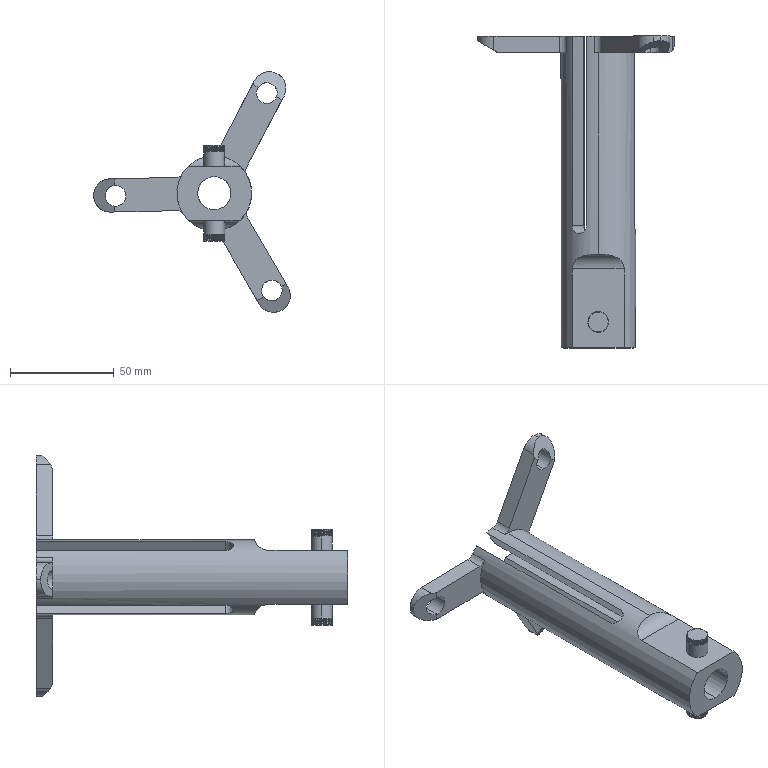Part | SolidWorks | features ICE 5, Fillet 2, SweepThread 2, Chamfer 1, Cut 1, Revolution 1 | 1 solid | 102 faces | box 94.58 x 150 x 115.79 mm | volume 107737 mm3 | cylinder 66 | plane 30 | spline 6 | commonest cylinder face diameters 10 x40 8 x13 16 x9 14.8 x2 36 x2